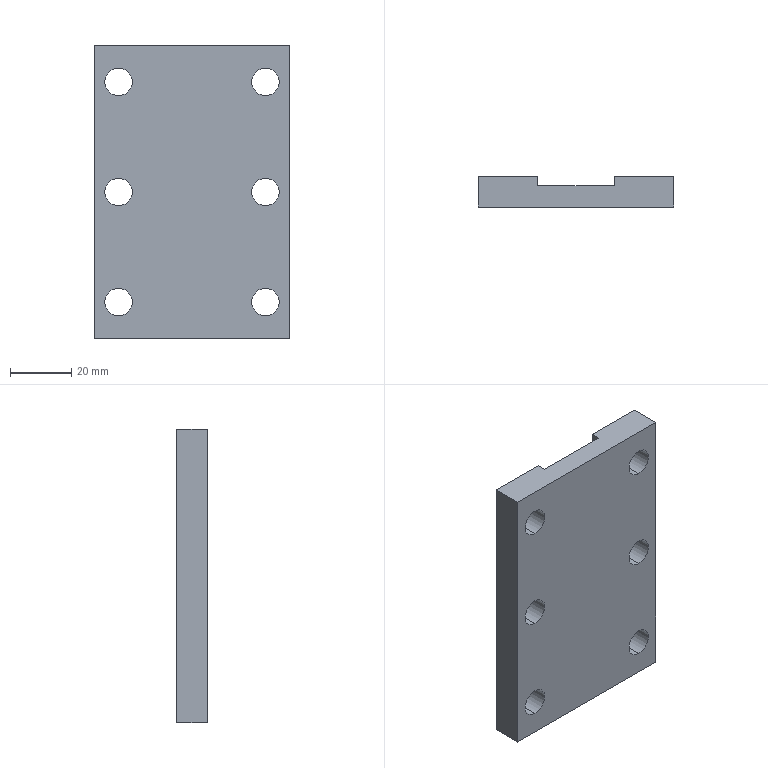Part | STEP file | 0245_213_Clamp | 1 solid | 22 faces | box 64 x 10 x 96 mm | volume 50375 mm3 | cylinder 12 | plane 10 | commonest cylinder face diameters 9 x12